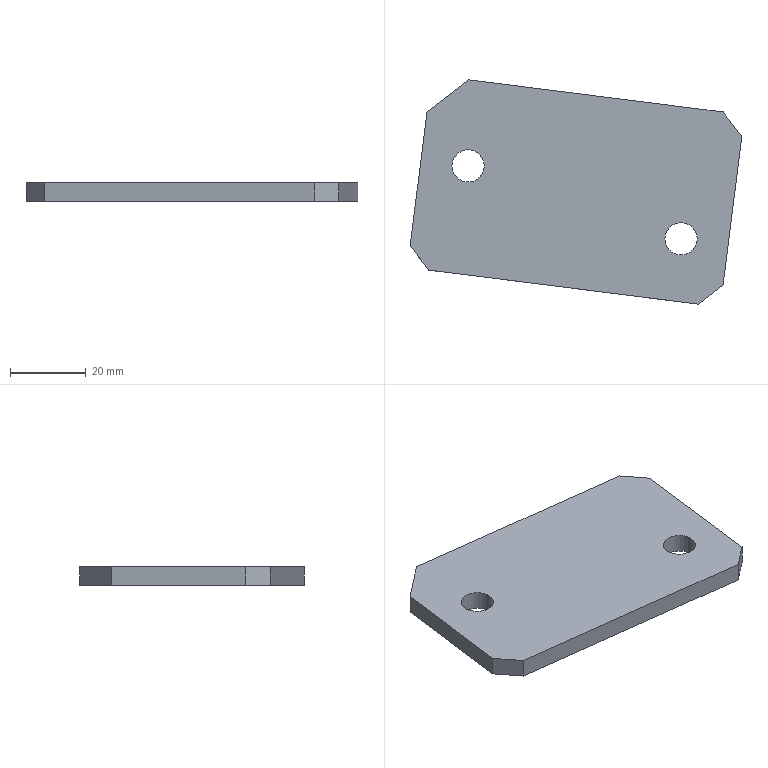Part | STEP file | gslz 2016.10.28-13_id1706_x_t | 1 solid | 12 faces | box 87.307 x 59.069 x 5 mm | volume 20118 mm3 | plane 10 | cylinder 2 | commonest cylinder face diameters 8.5 x2
STEP:
#1=CARTESIAN_POINT('',(0.,0.,0.));
#2=DIRECTION('',(0.,0.,1.));
#3=DIRECTION('',(1.,0.,0.));
#4=AXIS2_PLACEMENT_3D('',#1,#2,#3);
#5=CARTESIAN_POINT('',(33.844,160.175,-99.));
#6=VERTEX_POINT('',#5);
#7=CARTESIAN_POINT('',(-37.177,169.147,-99.));
#8=VERTEX_POINT('',#7);
#9=CARTESIAN_POINT('',(-1593.802,365.794,-99.));
#10=DIRECTION('',(-0.9921,0.1253,0.));
#11=VECTOR('',#10,1.);
#12=LINE('',#9,#11);
#13=CARTESIAN_POINT('',(-1593.802,365.794,-99.));
#14=DIRECTION('',(0.1253,0.9921,0.));
#15=DIRECTION('',(-0.9921,0.1253,0.));
#16=AXIS2_PLACEMENT_3D('',#13,#14,#15);
#17=PLANE('',#16);
#18=CARTESIAN_POINT('',(0.,0.));
#19=DIRECTION('',(1.,0.));
#20=VECTOR('',#19,1.);
#21=LINE('',#18,#20);
#22=(GEOMETRIC_REPRESENTATION_CONTEXT(2)PARAMETRIC_REPRESENTATION_CONTEXT()REPRESENTATION_CONTEXT('',''));
#23=DEFINITIONAL_REPRESENTATION('',(#21),#22);
#24=PCURVE('',#17,#23);
#25=CARTESIAN_POINT('',(-1586.721,421.848,-99.));
#26=DIRECTION('',(0.,0.,1.));
#27=DIRECTION('',(1.,0.,0.));
#28=AXIS2_PLACEMENT_3D('',#25,#26,#27);
#29=PLANE('',#28);
#30=CARTESIAN_POINT('',(-7.081,-56.054));
#31=DIRECTION('',(-0.9921,0.1253));
#32=VECTOR('',#31,1.);
#33=LINE('',#30,#32);
#34=(GEOMETRIC_REPRESENTATION_CONTEXT(2)PARAMETRIC_REPRESENTATION_CONTEXT()REPRESENTATION_CONTEXT('',''));
#35=DEFINITIONAL_REPRESENTATION('',(#33),#34);
#36=PCURVE('',#29,#35);
#37=SURFACE_CURVE('',#12,(#24,#36),.PCURVE_S1.);
#38=EDGE_CURVE('',#6,#8,#37,.T.);
#39=ORIENTED_EDGE('',*,*,#38,.F.);
#40=CARTESIAN_POINT('',(33.844,160.175,-94.));
#41=VERTEX_POINT('',#40);
#42=CARTESIAN_POINT('',(33.844,160.175,-99.));
#43=DIRECTION('',(0.,0.,1.));
#44=VECTOR('',#43,1.);
#45=LINE('',#42,#44);
#46=CARTESIAN_POINT('',(-1640.583,0.));
#47=DIRECTION('',(0.,1.));
#48=VECTOR('',#47,1.);
#49=LINE('',#46,#48);
#50=(GEOMETRIC_REPRESENTATION_CONTEXT(2)PARAMETRIC_REPRESENTATION_CONTEXT()REPRESENTATION_CONTEXT('',''));
#51=DEFINITIONAL_REPRESENTATION('',(#49),#50);
#52=PCURVE('',#17,#51);
#53=CARTESIAN_POINT('',(33.681,160.048,-99.));
#54=DIRECTION('',(-0.6129,0.7902,0.));
#55=DIRECTION('',(0.,0.,1.));
#56=AXIS2_PLACEMENT_3D('',#53,#54,#55);
#57=PLANE('',#56);
#58=CARTESIAN_POINT('',(0.,0.2071));
#59=DIRECTION('',(1.,0.));
#60=VECTOR('',#59,1.);
#61=LINE('',#58,#60);
#62=(GEOMETRIC_REPRESENTATION_CONTEXT(2)PARAMETRIC_REPRESENTATION_CONTEXT()REPRESENTATION_CONTEXT('',''));
#63=DEFINITIONAL_REPRESENTATION('',(#61),#62);
#64=PCURVE('',#57,#63);
#65=SURFACE_CURVE('',#45,(#52,#64),.PCURVE_S1.);
#66=EDGE_CURVE('',#6,#41,#65,.T.);
#67=ORIENTED_EDGE('',*,*,#66,.T.);
#68=CARTESIAN_POINT('',(-37.177,169.147,-94.));
#69=VERTEX_POINT('',#68);
#70=CARTESIAN_POINT('',(-1593.802,365.794,-94.));
#71=DIRECTION('',(-0.9921,0.1253,0.));
#72=VECTOR('',#71,1.);
#73=LINE('',#70,#72);
#74=CARTESIAN_POINT('',(0.,5.));
#75=DIRECTION('',(1.,0.));
#76=VECTOR('',#75,1.);
#77=LINE('',#74,#76);
#78=(GEOMETRIC_REPRESENTATION_CONTEXT(2)PARAMETRIC_REPRESENTATION_CONTEXT()REPRESENTATION_CONTEXT('',''));
#79=DEFINITIONAL_REPRESENTATION('',(#77),#78);
#80=PCURVE('',#17,#79);
#81=CARTESIAN_POINT('',(-1586.721,421.848,-94.));
#82=DIRECTION('',(0.,0.,1.));
#83=DIRECTION('',(1.,0.,0.));
#84=AXIS2_PLACEMENT_3D('',#81,#82,#83);
#85=PLANE('',#84);
#86=CARTESIAN_POINT('',(-7.081,-56.054));
#87=DIRECTION('',(-0.9921,0.1253));
#88=VECTOR('',#87,1.);
#89=LINE('',#86,#88);
#90=(GEOMETRIC_REPRESENTATION_CONTEXT(2)PARAMETRIC_REPRESENTATION_CONTEXT()REPRESENTATION_CONTEXT('',''));
#91=DEFINITIONAL_REPRESENTATION('',(#89),#90);
#92=PCURVE('',#85,#91);
#93=SURFACE_CURVE('',#73,(#80,#92),.PCURVE_S1.);
#94=EDGE_CURVE('',#41,#69,#93,.T.);
#95=ORIENTED_EDGE('',*,*,#94,.T.);
#96=CARTESIAN_POINT('',(-37.177,169.147,-99.));
#97=DIRECTION('',(0.,0.,-1.));
#98=VECTOR('',#97,1.);
#99=LINE('',#96,#98);
#100=CARTESIAN_POINT('',(-1568.997,0.));
#101=DIRECTION('',(0.,-1.));
#102=VECTOR('',#101,1.);
#103=LINE('',#100,#102);
#104=(GEOMETRIC_REPRESENTATION_CONTEXT(2)PARAMETRIC_REPRESENTATION_CONTEXT()REPRESENTATION_CONTEXT('',''));
#105=DEFINITIONAL_REPRESENTATION('',(#103),#104);
#106=PCURVE('',#17,#105);
#107=CARTESIAN_POINT('',(-42.251,175.688,-99.));
#108=DIRECTION('',(-0.7902,-0.6129,0.));
#109=DIRECTION('',(0.,0.,-1.));
#110=AXIS2_PLACEMENT_3D('',#107,#108,#109);
#111=PLANE('',#110);
#112=CARTESIAN_POINT('',(0.,8.278));
#113=DIRECTION('',(1.,0.));
#114=VECTOR('',#113,1.);
#115=LINE('',#112,#114);
#116=(GEOMETRIC_REPRESENTATION_CONTEXT(2)PARAMETRIC_REPRESENTATION_CONTEXT()REPRESENTATION_CONTEXT('',''));
#117=DEFINITIONAL_REPRESENTATION('',(#115),#116);
#118=PCURVE('',#111,#117);
#119=SURFACE_CURVE('',#99,(#106,#118),.PCURVE_S1.);
#120=EDGE_CURVE('',#69,#8,#119,.T.);
#121=ORIENTED_EDGE('',*,*,#120,.T.);
#122=EDGE_LOOP('',(#39,#67,#95,#121));
#123=FACE_BOUND('',#122,.T.);
#124=ADVANCED_FACE('',(#123),#17,.F.);
#125=CARTESIAN_POINT('',(-37.664,210.829,-94.));
#126=VERTEX_POINT('',#125);
#127=CARTESIAN_POINT('',(-42.124,175.524,-94.));
#128=VERTEX_POINT('',#127);
#129=CARTESIAN_POINT('',(-35.758,225.916,-94.));
#130=DIRECTION('',(-0.1253,-0.9921,0.));
#131=VECTOR('',#130,1.);
#132=LINE('',#129,#131);
#133=CARTESIAN_POINT('',(-35.758,225.916,-99.));
#134=DIRECTION('',(-0.9921,0.1253,0.));
#135=DIRECTION('',(-0.1253,-0.9921,0.));
#136=AXIS2_PLACEMENT_3D('',#133,#134,#135);
#137=PLANE('',#136);
#138=CARTESIAN_POINT('',(0.,5.));
#139=DIRECTION('',(1.,0.));
#140=VECTOR('',#139,1.);
#141=LINE('',#138,#140);
#142=(GEOMETRIC_REPRESENTATION_CONTEXT(2)PARAMETRIC_REPRESENTATION_CONTEXT()REPRESENTATION_CONTEXT('',''));
#143=DEFINITIONAL_REPRESENTATION('',(#141),#142);
#144=PCURVE('',#137,#143);
#145=CARTESIAN_POINT('',(1550.963,-195.932));
#146=DIRECTION('',(-0.1253,-0.9921));
#147=VECTOR('',#146,1.);
#148=LINE('',#145,#147);
#149=(GEOMETRIC_REPRESENTATION_CONTEXT(2)PARAMETRIC_REPRESENTATION_CONTEXT()REPRESENTATION_CONTEXT('',''));
#150=DEFINITIONAL_REPRESENTATION('',(#148),#149);
#151=PCURVE('',#85,#150);
#152=SURFACE_CURVE('',#132,(#144,#151),.PCURVE_S1.);
#153=EDGE_CURVE('',#126,#128,#152,.T.);
#154=ORIENTED_EDGE('',*,*,#153,.F.);
#155=CARTESIAN_POINT('',(-37.664,210.829,-99.));
#156=VERTEX_POINT('',#155);
#157=CARTESIAN_POINT('',(-37.664,210.829,-99.));
#158=DIRECTION('',(0.,0.,-1.));
#159=VECTOR('',#158,1.);
#160=LINE('',#157,#159);
#161=CARTESIAN_POINT('',(15.207,0.));
#162=DIRECTION('',(0.,-1.));
#163=VECTOR('',#162,1.);
#164=LINE('',#161,#163);
#165=(GEOMETRIC_REPRESENTATION_CONTEXT(2)PARAMETRIC_REPRESENTATION_CONTEXT()REPRESENTATION_CONTEXT('',''));
#166=DEFINITIONAL_REPRESENTATION('',(#164),#165);
#167=PCURVE('',#137,#166);
#168=CARTESIAN_POINT('',(-26.653,219.37,-99.));
#169=DIRECTION('',(0.6129,-0.7902,0.));
#170=DIRECTION('',(0.,0.,1.));
#171=AXIS2_PLACEMENT_3D('',#168,#169,#170);
#172=PLANE('',#171);
#173=CARTESIAN_POINT('',(0.,13.935));
#174=DIRECTION('',(-1.,0.));
#175=VECTOR('',#174,1.);
#176=LINE('',#173,#175);
#177=(GEOMETRIC_REPRESENTATION_CONTEXT(2)PARAMETRIC_REPRESENTATION_CONTEXT()REPRESENTATION_CONTEXT('',''));
#178=DEFINITIONAL_REPRESENTATION('',(#176),#177);
#179=PCURVE('',#172,#178);
#180=SURFACE_CURVE('',#160,(#167,#179),.PCURVE_S1.);
#181=EDGE_CURVE('',#126,#156,#180,.T.);
#182=ORIENTED_EDGE('',*,*,#181,.T.);
#183=CARTESIAN_POINT('',(-42.124,175.524,-99.));
#184=VERTEX_POINT('',#183);
#185=CARTESIAN_POINT('',(-35.758,225.916,-99.));
#186=DIRECTION('',(-0.1253,-0.9921,0.));
#187=VECTOR('',#186,1.);
#188=LINE('',#185,#187);
#189=CARTESIAN_POINT('',(0.,0.));
#190=DIRECTION('',(1.,0.));
#191=VECTOR('',#190,1.);
#192=LINE('',#189,#191);
#193=(GEOMETRIC_REPRESENTATION_CONTEXT(2)PARAMETRIC_REPRESENTATION_CONTEXT()REPRESENTATION_CONTEXT('',''));
#194=DEFINITIONAL_REPRESENTATION('',(#192),#193);
#195=PCURVE('',#137,#194);
#196=CARTESIAN_POINT('',(1550.963,-195.932));
#197=DIRECTION('',(-0.1253,-0.9921));
#198=VECTOR('',#197,1.);
#199=LINE('',#196,#198);
#200=(GEOMETRIC_REPRESENTATION_CONTEXT(2)PARAMETRIC_REPRESENTATION_CONTEXT()REPRESENTATION_CONTEXT('',''));
#201=DEFINITIONAL_REPRESENTATION('',(#199),#200);
#202=PCURVE('',#29,#201);
#203=SURFACE_CURVE('',#188,(#195,#202),.PCURVE_S1.);
#204=EDGE_CURVE('',#156,#184,#203,.T.);
#205=ORIENTED_EDGE('',*,*,#204,.T.);
#206=CARTESIAN_POINT('',(-42.124,175.524,-99.));
#207=DIRECTION('',(0.,0.,1.));
#208=VECTOR('',#207,1.);
#209=LINE('',#206,#208);
#210=CARTESIAN_POINT('',(50.793,0.));
#211=DIRECTION('',(0.,1.));
#212=VECTOR('',#211,1.);
#213=LINE('',#210,#212);
#214=(GEOMETRIC_REPRESENTATION_CONTEXT(2)PARAMETRIC_REPRESENTATION_CONTEXT()REPRESENTATION_CONTEXT('',''));
#215=DEFINITIONAL_REPRESENTATION('',(#213),#214);
#216=PCURVE('',#137,#215);
#217=CARTESIAN_POINT('',(0.,0.2071));
#218=DIRECTION('',(-1.,0.));
#219=VECTOR('',#218,1.);
#220=LINE('',#217,#219);
#221=(GEOMETRIC_REPRESENTATION_CONTEXT(2)PARAMETRIC_REPRESENTATION_CONTEXT()REPRESENTATION_CONTEXT('',''));
#222=DEFINITIONAL_REPRESENTATION('',(#220),#221);
#223=PCURVE('',#111,#222);
#224=SURFACE_CURVE('',#209,(#216,#223),.PCURVE_S1.);
#225=EDGE_CURVE('',#184,#128,#224,.T.);
#226=ORIENTED_EDGE('',*,*,#225,.T.);
#227=EDGE_LOOP('',(#154,#182,#205,#226));
#228=FACE_BOUND('',#227,.T.);
#229=ADVANCED_FACE('',(#228),#137,.T.);
#230=CARTESIAN_POINT('',(40.236,210.772,-99.));
#231=VERTEX_POINT('',#230);
#232=CARTESIAN_POINT('',(-26.816,219.243,-99.));
#233=VERTEX_POINT('',#232);
#234=CARTESIAN_POINT('',(-1587.41,416.392,-99.));
#235=DIRECTION('',(-0.9921,0.1253,0.));
#236=VECTOR('',#235,1.);
#237=LINE('',#234,#236);
#238=CARTESIAN_POINT('',(-1587.41,416.392,-99.));
#239=DIRECTION('',(0.1253,0.9921,0.));
#240=DIRECTION('',(-0.9921,0.1253,0.));
#241=AXIS2_PLACEMENT_3D('',#238,#239,#240);
#242=PLANE('',#241);
#243=CARTESIAN_POINT('',(0.,0.));
#244=DIRECTION('',(1.,0.));
#245=VECTOR('',#244,1.);
#246=LINE('',#243,#245);
#247=(GEOMETRIC_REPRESENTATION_CONTEXT(2)PARAMETRIC_REPRESENTATION_CONTEXT()REPRESENTATION_CONTEXT('',''));
#248=DEFINITIONAL_REPRESENTATION('',(#246),#247);
#249=PCURVE('',#242,#248);
#250=CARTESIAN_POINT('',(-0.6893,-5.457));
#251=DIRECTION('',(-0.9921,0.1253));
#252=VECTOR('',#251,1.);
#253=LINE('',#250,#252);
#254=(GEOMETRIC_REPRESENTATION_CONTEXT(2)PARAMETRIC_REPRESENTATION_CONTEXT()REPRESENTATION_CONTEXT('',''));
#255=DEFINITIONAL_REPRESENTATION('',(#253),#254);
#256=PCURVE('',#29,#255);
#257=SURFACE_CURVE('',#237,(#249,#256),.PCURVE_S1.);
#258=EDGE_CURVE('',#231,#233,#257,.T.);
#259=ORIENTED_EDGE('',*,*,#258,.T.);
#260=CARTESIAN_POINT('',(-26.816,219.243,-94.));
#261=VERTEX_POINT('',#260);
#262=CARTESIAN_POINT('',(-26.816,219.243,-99.));
#263=DIRECTION('',(0.,0.,1.));
#264=VECTOR('',#263,1.);
#265=LINE('',#262,#264);
#266=CARTESIAN_POINT('',(-1572.997,0.));
#267=DIRECTION('',(0.,1.));
#268=VECTOR('',#267,1.);
#269=LINE('',#266,#268);
#270=(GEOMETRIC_REPRESENTATION_CONTEXT(2)PARAMETRIC_REPRESENTATION_CONTEXT()REPRESENTATION_CONTEXT('',''));
#271=DEFINITIONAL_REPRESENTATION('',(#269),#270);
#272=PCURVE('',#242,#271);
#273=CARTESIAN_POINT('',(0.,0.2071));
#274=DIRECTION('',(1.,0.));
#275=VECTOR('',#274,1.);
#276=LINE('',#273,#275);
#277=(GEOMETRIC_REPRESENTATION_CONTEXT(2)PARAMETRIC_REPRESENTATION_CONTEXT()REPRESENTATION_CONTEXT('',''));
#278=DEFINITIONAL_REPRESENTATION('',(#276),#277);
#279=PCURVE('',#172,#278);
#280=SURFACE_CURVE('',#265,(#272,#279),.PCURVE_S1.);
#281=EDGE_CURVE('',#233,#261,#280,.T.);
#282=ORIENTED_EDGE('',*,*,#281,.T.);
#283=CARTESIAN_POINT('',(40.236,210.772,-94.));
#284=VERTEX_POINT('',#283);
#285=CARTESIAN_POINT('',(-1587.41,416.392,-94.));
#286=DIRECTION('',(-0.9921,0.1253,0.));
#287=VECTOR('',#286,1.);
#288=LINE('',#285,#287);
#289=CARTESIAN_POINT('',(0.,5.));
#290=DIRECTION('',(1.,0.));
#291=VECTOR('',#290,1.);
#292=LINE('',#289,#291);
#293=(GEOMETRIC_REPRESENTATION_CONTEXT(2)PARAMETRIC_REPRESENTATION_CONTEXT()REPRESENTATION_CONTEXT('',''));
#294=DEFINITIONAL_REPRESENTATION('',(#292),#293);
#295=PCURVE('',#242,#294);
#296=CARTESIAN_POINT('',(-0.6893,-5.457));
#297=DIRECTION('',(-0.9921,0.1253));
#298=VECTOR('',#297,1.);
#299=LINE('',#296,#298);
#300=(GEOMETRIC_REPRESENTATION_CONTEXT(2)PARAMETRIC_REPRESENTATION_CONTEXT()REPRESENTATION_CONTEXT('',''));
#301=DEFINITIONAL_REPRESENTATION('',(#299),#300);
#302=PCURVE('',#85,#301);
#303=SURFACE_CURVE('',#288,(#295,#302),.PCURVE_S1.);
#304=EDGE_CURVE('',#284,#261,#303,.T.);
#305=ORIENTED_EDGE('',*,*,#304,.F.);
#306=CARTESIAN_POINT('',(40.236,210.772,-99.));
#307=DIRECTION('',(0.,0.,-1.));
#308=VECTOR('',#307,1.);
#309=LINE('',#306,#308);
#310=CARTESIAN_POINT('',(-1640.583,0.));
#311=DIRECTION('',(0.,-1.));
#312=VECTOR('',#311,1.);
#313=LINE('',#310,#312);
#314=(GEOMETRIC_REPRESENTATION_CONTEXT(2)PARAMETRIC_REPRESENTATION_CONTEXT()REPRESENTATION_CONTEXT('',''));
#315=DEFINITIONAL_REPRESENTATION('',(#313),#314);
#316=PCURVE('',#242,#315);
#317=CARTESIAN_POINT('',(45.31,204.231,-99.));
#318=DIRECTION('',(0.7902,0.6129,0.));
#319=DIRECTION('',(0.,0.,-1.));
#320=AXIS2_PLACEMENT_3D('',#317,#318,#319);
#321=PLANE('',#320);
#322=CARTESIAN_POINT('',(0.,8.278));
#323=DIRECTION('',(1.,0.));
#324=VECTOR('',#323,1.);
#325=LINE('',#322,#324);
#326=(GEOMETRIC_REPRESENTATION_CONTEXT(2)PARAMETRIC_REPRESENTATION_CONTEXT()REPRESENTATION_CONTEXT('',''));
#327=DEFINITIONAL_REPRESENTATION('',(#325),#326);
#328=PCURVE('',#321,#327);
#329=SURFACE_CURVE('',#309,(#316,#328),.PCURVE_S1.);
#330=EDGE_CURVE('',#284,#231,#329,.T.);
#331=ORIENTED_EDGE('',*,*,#330,.T.);
#332=EDGE_LOOP('',(#259,#282,#305,#331));
#333=FACE_BOUND('',#332,.T.);
#334=ADVANCED_FACE('',(#333),#242,.T.);
#335=CARTESIAN_POINT('',(45.183,204.395,-99.));
#336=VERTEX_POINT('',#335);
#337=CARTESIAN_POINT('',(40.222,165.121,-99.));
#338=VERTEX_POINT('',#337);
#339=CARTESIAN_POINT('',(46.588,215.514,-99.));
#340=DIRECTION('',(-0.1253,-0.9921,0.));
#341=VECTOR('',#340,1.);
#342=LINE('',#339,#341);
#343=CARTESIAN_POINT('',(46.588,215.514,-99.));
#344=DIRECTION('',(-0.9921,0.1253,0.));
#345=DIRECTION('',(-0.1253,-0.9921,0.));
#346=AXIS2_PLACEMENT_3D('',#343,#344,#345);
#347=PLANE('',#346);
#348=CARTESIAN_POINT('',(0.,0.));
#349=DIRECTION('',(1.,0.));
#350=VECTOR('',#349,1.);
#351=LINE('',#348,#350);
#352=(GEOMETRIC_REPRESENTATION_CONTEXT(2)PARAMETRIC_REPRESENTATION_CONTEXT()REPRESENTATION_CONTEXT('',''));
#353=DEFINITIONAL_REPRESENTATION('',(#351),#352);
#354=PCURVE('',#347,#353);
#355=CARTESIAN_POINT('',(1633.309,-206.334));
#356=DIRECTION('',(-0.1253,-0.9921));
#357=VECTOR('',#356,1.);
#358=LINE('',#355,#357);
#359=(GEOMETRIC_REPRESENTATION_CONTEXT(2)PARAMETRIC_REPRESENTATION_CONTEXT()REPRESENTATION_CONTEXT('',''));
#360=DEFINITIONAL_REPRESENTATION('',(#358),#359);
#361=PCURVE('',#29,#360);
#362=SURFACE_CURVE('',#342,(#354,#361),.PCURVE_S1.);
#363=EDGE_CURVE('',#336,#338,#362,.T.);
#364=ORIENTED_EDGE('',*,*,#363,.F.);
#365=CARTESIAN_POINT('',(45.183,204.395,-94.));
#366=VERTEX_POINT('',#365);
#367=CARTESIAN_POINT('',(45.183,204.395,-99.));
#368=DIRECTION('',(0.,0.,1.));
#369=VECTOR('',#368,1.);
#370=LINE('',#367,#369);
#371=CARTESIAN_POINT('',(11.207,0.));
#372=DIRECTION('',(0.,1.));
#373=VECTOR('',#372,1.);
#374=LINE('',#371,#373);
#375=(GEOMETRIC_REPRESENTATION_CONTEXT(2)PARAMETRIC_REPRESENTATION_CONTEXT()REPRESENTATION_CONTEXT('',''));
#376=DEFINITIONAL_REPRESENTATION('',(#374),#375);
#377=PCURVE('',#347,#376);
#378=CARTESIAN_POINT('',(0.,0.2071));
#379=DIRECTION('',(-1.,0.));
#380=VECTOR('',#379,1.);
#381=LINE('',#378,#380);
#382=(GEOMETRIC_REPRESENTATION_CONTEXT(2)PARAMETRIC_REPRESENTATION_CONTEXT()REPRESENTATION_CONTEXT('',''));
#383=DEFINITIONAL_REPRESENTATION('',(#381),#382);
#384=PCURVE('',#321,#383);
#385=SURFACE_CURVE('',#370,(#377,#384),.PCURVE_S1.);
#386=EDGE_CURVE('',#336,#366,#385,.T.);
#387=ORIENTED_EDGE('',*,*,#386,.T.);
#388=CARTESIAN_POINT('',(40.222,165.121,-94.));
#389=VERTEX_POINT('',#388);
#390=CARTESIAN_POINT('',(46.588,215.514,-94.));
#391=DIRECTION('',(-0.1253,-0.9921,0.));
#392=VECTOR('',#391,1.);
#393=LINE('',#390,#392);
#394=CARTESIAN_POINT('',(0.,5.));
#395=DIRECTION('',(1.,0.));
#396=VECTOR('',#395,1.);
#397=LINE('',#394,#396);
#398=(GEOMETRIC_REPRESENTATION_CONTEXT(2)PARAMETRIC_REPRESENTATION_CONTEXT()REPRESENTATION_CONTEXT('',''));
#399=DEFINITIONAL_REPRESENTATION('',(#397),#398);
#400=PCURVE('',#347,#399);
#401=CARTESIAN_POINT('',(1633.309,-206.334));
#402=DIRECTION('',(-0.1253,-0.9921));
#403=VECTOR('',#402,1.);
#404=LINE('',#401,#403);
#405=(GEOMETRIC_REPRESENTATION_CONTEXT(2)PARAMETRIC_REPRESENTATION_CONTEXT()REPRESENTATION_CONTEXT('',''));
#406=DEFINITIONAL_REPRESENTATION('',(#404),#405);
#407=PCURVE('',#85,#406);
#408=SURFACE_CURVE('',#393,(#400,#407),.PCURVE_S1.);
#409=EDGE_CURVE('',#366,#389,#408,.T.);
#410=ORIENTED_EDGE('',*,*,#409,.T.);
#411=CARTESIAN_POINT('',(40.222,165.121,-99.));
#412=DIRECTION('',(0.,0.,-1.));
#413=VECTOR('',#412,1.);
#414=LINE('',#411,#413);
#415=CARTESIAN_POINT('',(50.793,0.));
#416=DIRECTION('',(0.,-1.));
#417=VECTOR('',#416,1.);
#418=LINE('',#415,#417);
#419=(GEOMETRIC_REPRESENTATION_CONTEXT(2)PARAMETRIC_REPRESENTATION_CONTEXT()REPRESENTATION_CONTEXT('',''));
#420=DEFINITIONAL_REPRESENTATION('',(#418),#419);
#421=PCURVE('',#347,#420);
#422=CARTESIAN_POINT('',(0.,8.278));
#423=DIRECTION('',(-1.,0.));
#424=VECTOR('',#423,1.);
#425=LINE('',#422,#424);
#426=(GEOMETRIC_REPRESENTATION_CONTEXT(2)PARAMETRIC_REPRESENTATION_CONTEXT()REPRESENTATION_CONTEXT('',''));
#427=DEFINITIONAL_REPRESENTATION('',(#425),#426);
#428=PCURVE('',#57,#427);
#429=SURFACE_CURVE('',#414,(#421,#428),.PCURVE_S1.);
#430=EDGE_CURVE('',#389,#338,#429,.T.);
#431=ORIENTED_EDGE('',*,*,#430,.T.);
#432=EDGE_LOOP('',(#364,#387,#410,#431));
#433=FACE_BOUND('',#432,.T.);
#434=ADVANCED_FACE('',(#433),#347,.F.);
#435=CARTESIAN_POINT('',(-31.116,196.571,-99.));
#436=VERTEX_POINT('',#435);
#437=CARTESIAN_POINT('',(-26.866,196.571,-99.));
#438=DIRECTION('',(0.,0.,-1.));
#439=DIRECTION('',(-1.,0.,0.));
#440=AXIS2_PLACEMENT_3D('',#437,#438,#439);
#441=CIRCLE('',#440,4.25);
#442=CARTESIAN_POINT('',(-26.866,196.571,-99.));
#443=DIRECTION('',(0.,0.,1.));
#444=DIRECTION('',(1.,0.,0.));
#445=AXIS2_PLACEMENT_3D('',#442,#443,#444);
#446=CYLINDRICAL_SURFACE('',#445,4.25);
#447=CARTESIAN_POINT('',(9.425,0.));
#448=DIRECTION('',(-1.,0.));
#449=VECTOR('',#448,1.);
#450=LINE('',#447,#449);
#451=(GEOMETRIC_REPRESENTATION_CONTEXT(2)PARAMETRIC_REPRESENTATION_CONTEXT()REPRESENTATION_CONTEXT('',''));
#452=DEFINITIONAL_REPRESENTATION('',(#450),#451);
#453=PCURVE('',#446,#452);
#454=CARTESIAN_POINT('',(1555.605,-225.278));
#455=CARTESIAN_POINT('',(1555.605,-217.916));
#456=CARTESIAN_POINT('',(1561.98,-221.597));
#457=CARTESIAN_POINT('',(1568.355,-225.278));
#458=CARTESIAN_POINT('',(1561.98,-228.958));
#459=CARTESIAN_POINT('',(1555.605,-232.639));
#460=CARTESIAN_POINT('',(1555.605,-225.278));
#461=(BOUNDED_CURVE()B_SPLINE_CURVE(2,(#454,#455,#456,#457,#458,#459,#460),.UNSPECIFIED.,.T.,.F.)B_SPLINE_CURVE_WITH_KNOTS((1,2,2,2,2,1),(-2.094,0.,2.094,4.189,6.283,8.378),.UNSPECIFIED.)CURVE()GEOMETRIC_REPRESENTATION_ITEM()RATIONAL_B_SPLINE_CURVE((1.,0.5,1.,0.5,1.,0.5,1.))REPRESENTATION_ITEM(''));
#462=(GEOMETRIC_REPRESENTATION_CONTEXT(2)PARAMETRIC_REPRESENTATION_CONTEXT()REPRESENTATION_CONTEXT('',''));
#463=DEFINITIONAL_REPRESENTATION('',(#461),#462);
#464=PCURVE('',#29,#463);
#465=SURFACE_CURVE('',#441,(#453,#464),.PCURVE_S1.);
#466=EDGE_CURVE('',#436,#436,#465,.T.);
#467=ORIENTED_EDGE('',*,*,#466,.F.);
#468=CARTESIAN_POINT('',(-31.116,196.571,-94.));
#469=VERTEX_POINT('',#468);
#470=CARTESIAN_POINT('',(-31.116,196.571,-99.));
#471=CARTESIAN_POINT('',(-31.116,196.571,-94.));
#472=B_SPLINE_CURVE_WITH_KNOTS('',1,(#470,#471),.UNSPECIFIED.,.F.,.F.,(2,2),(0.,5.),.PIECEWISE_BEZIER_KNOTS.);
#473=CARTESIAN_POINT('',(9.425,0.));
#474=DIRECTION('',(0.,1.));
#475=VECTOR('',#474,1.);
#476=LINE('',#473,#475);
#477=(GEOMETRIC_REPRESENTATION_CONTEXT(2)PARAMETRIC_REPRESENTATION_CONTEXT()REPRESENTATION_CONTEXT('',''));
#478=DEFINITIONAL_REPRESENTATION('',(#476),#477);
#479=PCURVE('',#446,#478);
#480=CARTESIAN_POINT('',(3.142,0.));
#481=DIRECTION('',(0.,1.));
#482=VECTOR('',#481,1.);
#483=LINE('',#480,#482);
#484=(GEOMETRIC_REPRESENTATION_CONTEXT(2)PARAMETRIC_REPRESENTATION_CONTEXT()REPRESENTATION_CONTEXT('',''));
#485=DEFINITIONAL_REPRESENTATION('',(#483),#484);
#486=PCURVE('',#446,#485);
#487=SEAM_CURVE('',#472,(#479,#486),.PCURVE_S1.);
#488=EDGE_CURVE('',#436,#469,#487,.T.);
#489=ORIENTED_EDGE('',*,*,#488,.T.);
#490=CARTESIAN_POINT('',(-26.866,196.571,-94.));
#491=DIRECTION('',(0.,0.,-1.));
#492=DIRECTION('',(-1.,0.,0.));
#493=AXIS2_PLACEMENT_3D('',#490,#491,#492);
#494=CIRCLE('',#493,4.25);
#495=CARTESIAN_POINT('',(9.425,5.));
#496=DIRECTION('',(-1.,0.));
#497=VECTOR('',#496,1.);
#498=LINE('',#495,#497);
#499=(GEOMETRIC_REPRESENTATION_CONTEXT(2)PARAMETRIC_REPRESENTATION_CONTEXT()REPRESENTATION_CONTEXT('',''));
#500=DEFINITIONAL_REPRESENTATION('',(#498),#499);
#501=PCURVE('',#446,#500);
#502=CARTESIAN_POINT('',(1555.605,-225.278));
#503=CARTESIAN_POINT('',(1555.605,-217.916));
#504=CARTESIAN_POINT('',(1561.98,-221.597));
#505=CARTESIAN_POINT('',(1568.355,-225.278));
#506=CARTESIAN_POINT('',(1561.98,-228.958));
#507=CARTESIAN_POINT('',(1555.605,-232.639));
#508=CARTESIAN_POINT('',(1555.605,-225.278));
#509=(BOUNDED_CURVE()B_SPLINE_CURVE(2,(#502,#503,#504,#505,#506,#507,#508),.UNSPECIFIED.,.T.,.F.)B_SPLINE_CURVE_WITH_KNOTS((1,2,2,2,2,1),(-2.094,0.,2.094,4.189,6.283,8.378),.UNSPECIFIED.)CURVE()GEOMETRIC_REPRESENTATION_ITEM()RATIONAL_B_SPLINE_CURVE((1.,0.5,1.,0.5,1.,0.5,1.))REPRESENTATION_ITEM(''));
#510=(GEOMETRIC_REPRESENTATION_CONTEXT(2)PARAMETRIC_REPRESENTATION_CONTEXT()REPRESENTATION_CONTEXT('',''));
#511=DEFINITIONAL_REPRESENTATION('',(#509),#510);
#512=PCURVE('',#85,#511);
#513=SURFACE_CURVE('',#494,(#501,#512),.PCURVE_S1.);
#514=EDGE_CURVE('',#469,#469,#513,.T.);
#515=ORIENTED_EDGE('',*,*,#514,.T.);
#516=ORIENTED_EDGE('',*,*,#488,.F.);
#517=EDGE_LOOP('',(#467,#489,#515,#516));
#518=FACE_BOUND('',#517,.F.);
#519=ADVANCED_FACE('',(#518),#446,.F.);
#520=CARTESIAN_POINT('',(24.923,177.396,-99.));
#521=VERTEX_POINT('',#520);
#522=CARTESIAN_POINT('',(29.173,177.396,-99.));
#523=DIRECTION('',(0.,0.,-1.));
#524=DIRECTION('',(-1.,0.,0.));
#525=AXIS2_PLACEMENT_3D('',#522,#523,#524);
#526=CIRCLE('',#525,4.25);
#527=CARTESIAN_POINT('',(29.173,177.396,-99.));
#528=DIRECTION('',(0.,0.,1.));
#529=DIRECTION('',(1.,0.,0.));
#530=AXIS2_PLACEMENT_3D('',#527,#528,#529);
#531=CYLINDRICAL_SURFACE('',#530,4.25);
#532=CARTESIAN_POINT('',(9.425,0.));
#533=DIRECTION('',(-1.,0.));
#534=VECTOR('',#533,1.);
#535=LINE('',#532,#534);
#536=(GEOMETRIC_REPRESENTATION_CONTEXT(2)PARAMETRIC_REPRESENTATION_CONTEXT()REPRESENTATION_CONTEXT('',''));
#537=DEFINITIONAL_REPRESENTATION('',(#535),#536);
#538=PCURVE('',#531,#537);
#539=CARTESIAN_POINT('',(1611.644,-244.452));
#540=CARTESIAN_POINT('',(1611.644,-237.091));
#541=CARTESIAN_POINT('',(1618.019,-240.772));
#542=CARTESIAN_POINT('',(1624.394,-244.452));
#543=CARTESIAN_POINT('',(1618.019,-248.133));
#544=CARTESIAN_POINT('',(1611.644,-251.814));
#545=CARTESIAN_POINT('',(1611.644,-244.452));
#546=(BOUNDED_CURVE()B_SPLINE_CURVE(2,(#539,#540,#541,#542,#543,#544,#545),.UNSPECIFIED.,.T.,.F.)B_SPLINE_CURVE_WITH_KNOTS((1,2,2,2,2,1),(-2.094,0.,2.094,4.189,6.283,8.378),.UNSPECIFIED.)CURVE()GEOMETRIC_REPRESENTATION_ITEM()RATIONAL_B_SPLINE_CURVE((1.,0.5,1.,0.5,1.,0.5,1.))REPRESENTATION_ITEM(''));
#547=(GEOMETRIC_REPRESENTATION_CONTEXT(2)PARAMETRIC_REPRESENTATION_CONTEXT()REPRESENTATION_CONTEXT('',''));
#548=DEFINITIONAL_REPRESENTATION('',(#546),#547);
#549=PCURVE('',#29,#548);
#550=SURFACE_CURVE('',#526,(#538,#549),.PCURVE_S1.);
#551=EDGE_CURVE('',#521,#521,#550,.T.);
#552=ORIENTED_EDGE('',*,*,#551,.F.);
#553=CARTESIAN_POINT('',(24.923,177.396,-94.));
#554=VERTEX_POINT('',#553);
#555=CARTESIAN_POINT('',(24.923,177.396,-99.));
#556=CARTESIAN_POINT('',(24.923,177.396,-94.));
#557=B_SPLINE_CURVE_WITH_KNOTS('',1,(#555,#556),.UNSPECIFIED.,.F.,.F.,(2,2),(0.,5.),.PIECEWISE_BEZIER_KNOTS.);
#558=CARTESIAN_POINT('',(9.425,0.));
#559=DIRECTION('',(0.,1.));
#560=VECTOR('',#559,1.);
#561=LINE('',#558,#560);
#562=(GEOMETRIC_REPRESENTATION_CONTEXT(2)PARAMETRIC_REPRESENTATION_CONTEXT()REPRESENTATION_CONTEXT('',''));
#563=DEFINITIONAL_REPRESENTATION('',(#561),#562);
#564=PCURVE('',#531,#563);
#565=CARTESIAN_POINT('',(3.142,0.));
#566=DIRECTION('',(0.,1.));
#567=VECTOR('',#566,1.);
#568=LINE('',#565,#567);
#569=(GEOMETRIC_REPRESENTATION_CONTEXT(2)PARAMETRIC_REPRESENTATION_CONTEXT()REPRESENTATION_CONTEXT('',''));
#570=DEFINITIONAL_REPRESENTATION('',(#568),#569);
#571=PCURVE('',#531,#570);
#572=SEAM_CURVE('',#557,(#564,#571),.PCURVE_S1.);
#573=EDGE_CURVE('',#521,#554,#572,.T.);
#574=ORIENTED_EDGE('',*,*,#573,.T.);
#575=CARTESIAN_POINT('',(29.173,177.396,-94.));
#576=DIRECTION('',(0.,0.,-1.));
#577=DIRECTION('',(-1.,0.,0.));
#578=AXIS2_PLACEMENT_3D('',#575,#576,#577);
#579=CIRCLE('',#578,4.25);
#580=CARTESIAN_POINT('',(9.425,5.));
#581=DIRECTION('',(-1.,0.));
#582=VECTOR('',#581,1.);
#583=LINE('',#580,#582);
#584=(GEOMETRIC_REPRESENTATION_CONTEXT(2)PARAMETRIC_REPRESENTATION_CONTEXT()REPRESENTATION_CONTEXT('',''));
#585=DEFINITIONAL_REPRESENTATION('',(#583),#584);
#586=PCURVE('',#531,#585);
#587=CARTESIAN_POINT('',(1611.644,-244.452));
#588=CARTESIAN_POINT('',(1611.644,-237.091));
#589=CARTESIAN_POINT('',(1618.019,-240.772));
#590=CARTESIAN_POINT('',(1624.394,-244.452));
#591=CARTESIAN_POINT('',(1618.019,-248.133));
#592=CARTESIAN_POINT('',(1611.644,-251.814));
#593=CARTESIAN_POINT('',(1611.644,-244.452));
#594=(BOUNDED_CURVE()B_SPLINE_CURVE(2,(#587,#588,#589,#590,#591,#592,#593),.UNSPECIFIED.,.T.,.F.)B_SPLINE_CURVE_WITH_KNOTS((1,2,2,2,2,1),(-2.094,0.,2.094,4.189,6.283,8.378),.UNSPECIFIED.)CURVE()GEOMETRIC_REPRESENTATION_ITEM()RATIONAL_B_SPLINE_CURVE((1.,0.5,1.,0.5,1.,0.5,1.))REPRESENTATION_ITEM(''));
#595=(GEOMETRIC_REPRESENTATION_CONTEXT(2)PARAMETRIC_REPRESENTATION_CONTEXT()REPRESENTATION_CONTEXT('',''));
#596=DEFINITIONAL_REPRESENTATION('',(#594),#595);
#597=PCURVE('',#85,#596);
#598=SURFACE_CURVE('',#579,(#586,#597),.PCURVE_S1.);
#599=EDGE_CURVE('',#554,#554,#598,.T.);
#600=ORIENTED_EDGE('',*,*,#599,.T.);
#601=ORIENTED_EDGE('',*,*,#573,.F.);
#602=EDGE_LOOP('',(#552,#574,#600,#601));
#603=FACE_BOUND('',#602,.F.);
#604=ADVANCED_FACE('',(#603),#531,.F.);
#605=ORIENTED_EDGE('',*,*,#204,.F.);
#606=CARTESIAN_POINT('',(-26.653,219.37,-99.));
#607=DIRECTION('',(0.7902,0.6129,0.));
#608=VECTOR('',#607,1.);
#609=LINE('',#606,#608);
#610=CARTESIAN_POINT('',(1560.068,-202.478));
#611=DIRECTION('',(0.7902,0.6129));
#612=VECTOR('',#611,1.);
#613=LINE('',#610,#612);
#614=(GEOMETRIC_REPRESENTATION_CONTEXT(2)PARAMETRIC_REPRESENTATION_CONTEXT()REPRESENTATION_CONTEXT('',''));
#615=DEFINITIONAL_REPRESENTATION('',(#613),#614);
#616=PCURVE('',#29,#615);
#617=CARTESIAN_POINT('',(0.,0.));
#618=DIRECTION('',(0.,-1.));
#619=VECTOR('',#618,1.);
#620=LINE('',#617,#619);
#621=(GEOMETRIC_REPRESENTATION_CONTEXT(2)PARAMETRIC_REPRESENTATION_CONTEXT()REPRESENTATION_CONTEXT('',''));
#622=DEFINITIONAL_REPRESENTATION('',(#620),#621);
#623=PCURVE('',#172,#622);
#624=SURFACE_CURVE('',#609,(#616,#623),.PCURVE_S1.);
#625=EDGE_CURVE('',#156,#233,#624,.T.);
#626=ORIENTED_EDGE('',*,*,#625,.T.);
#627=ORIENTED_EDGE('',*,*,#258,.F.);
#628=CARTESIAN_POINT('',(45.31,204.231,-99.));
#629=DIRECTION('',(0.6129,-0.7902,0.));
#630=VECTOR('',#629,1.);
#631=LINE('',#628,#630);
#632=CARTESIAN_POINT('',(1632.031,-217.617));
#633=DIRECTION('',(0.6129,-0.7902));
#634=VECTOR('',#633,1.);
#635=LINE('',#632,#634);
#636=(GEOMETRIC_REPRESENTATION_CONTEXT(2)PARAMETRIC_REPRESENTATION_CONTEXT()REPRESENTATION_CONTEXT('',''));
#637=DEFINITIONAL_REPRESENTATION('',(#635),#636);
#638=PCURVE('',#29,#637);
#639=CARTESIAN_POINT('',(0.,0.));
#640=DIRECTION('',(0.,-1.));
#641=VECTOR('',#640,1.);
#642=LINE('',#639,#641);
#643=(GEOMETRIC_REPRESENTATION_CONTEXT(2)PARAMETRIC_REPRESENTATION_CONTEXT()REPRESENTATION_CONTEXT('',''));
#644=DEFINITIONAL_REPRESENTATION('',(#642),#643);
#645=PCURVE('',#321,#644);
#646=SURFACE_CURVE('',#631,(#638,#645),.PCURVE_S1.);
#647=EDGE_CURVE('',#231,#336,#646,.T.);
#648=ORIENTED_EDGE('',*,*,#647,.T.);
#649=ORIENTED_EDGE('',*,*,#363,.T.);
#650=CARTESIAN_POINT('',(33.681,160.048,-99.));
#651=DIRECTION('',(-0.7902,-0.6129,0.));
#652=VECTOR('',#651,1.);
#653=LINE('',#650,#652);
#654=CARTESIAN_POINT('',(1620.402,-261.801));
#655=DIRECTION('',(-0.7902,-0.6129));
#656=VECTOR('',#655,1.);
#657=LINE('',#654,#656);
#658=(GEOMETRIC_REPRESENTATION_CONTEXT(2)PARAMETRIC_REPRESENTATION_CONTEXT()REPRESENTATION_CONTEXT('',''));
#659=DEFINITIONAL_REPRESENTATION('',(#657),#658);
#660=PCURVE('',#29,#659);
#661=CARTESIAN_POINT('',(0.,0.));
#662=DIRECTION('',(0.,-1.));
#663=VECTOR('',#662,1.);
#664=LINE('',#661,#663);
#665=(GEOMETRIC_REPRESENTATION_CONTEXT(2)PARAMETRIC_REPRESENTATION_CONTEXT()REPRESENTATION_CONTEXT('',''));
#666=DEFINITIONAL_REPRESENTATION('',(#664),#665);
#667=PCURVE('',#57,#666);
#668=SURFACE_CURVE('',#653,(#660,#667),.PCURVE_S1.);
#669=EDGE_CURVE('',#338,#6,#668,.T.);
#670=ORIENTED_EDGE('',*,*,#669,.T.);
#671=ORIENTED_EDGE('',*,*,#38,.T.);
#672=CARTESIAN_POINT('',(-42.251,175.688,-99.));
#673=DIRECTION('',(-0.6129,0.7902,0.));
#674=VECTOR('',#673,1.);
#675=LINE('',#672,#674);
#676=CARTESIAN_POINT('',(1544.47,-246.161));
#677=DIRECTION('',(-0.6129,0.7902));
#678=VECTOR('',#677,1.);
#679=LINE('',#676,#678);
#680=(GEOMETRIC_REPRESENTATION_CONTEXT(2)PARAMETRIC_REPRESENTATION_CONTEXT()REPRESENTATION_CONTEXT('',''));
#681=DEFINITIONAL_REPRESENTATION('',(#679),#680);
#682=PCURVE('',#29,#681);
#683=CARTESIAN_POINT('',(0.,0.));
#684=DIRECTION('',(0.,-1.));
#685=VECTOR('',#684,1.);
#686=LINE('',#683,#685);
#687=(GEOMETRIC_REPRESENTATION_CONTEXT(2)PARAMETRIC_REPRESENTATION_CONTEXT()REPRESENTATION_CONTEXT('',''));
#688=DEFINITIONAL_REPRESENTATION('',(#686),#687);
#689=PCURVE('',#111,#688);
#690=SURFACE_CURVE('',#675,(#682,#689),.PCURVE_S1.);
#691=EDGE_CURVE('',#8,#184,#690,.T.);
#692=ORIENTED_EDGE('',*,*,#691,.T.);
#693=EDGE_LOOP('',(#605,#626,#627,#648,#649,#670,#671,#692));
#694=FACE_BOUND('',#693,.T.);
#695=ORIENTED_EDGE('',*,*,#466,.F.);
#696=EDGE_LOOP('',(#695));
#697=FACE_BOUND('',#696,.T.);
#698=ORIENTED_EDGE('',*,*,#551,.F.);
#699=EDGE_LOOP('',(#698));
#700=FACE_BOUND('',#699,.T.);
#701=ADVANCED_FACE('',(#694,#697,#700),#29,.F.);
#702=ORIENTED_EDGE('',*,*,#304,.T.);
#703=CARTESIAN_POINT('',(-902.615,-460.096,-94.));
#704=DIRECTION('',(-0.7902,-0.6129,0.));
#705=VECTOR('',#704,1.);
#706=LINE('',#703,#705);
#707=CARTESIAN_POINT('',(684.106,-881.944));
#708=DIRECTION('',(-0.7902,-0.6129));
#709=VECTOR('',#708,1.);
#710=LINE('',#707,#709);
#711=(GEOMETRIC_REPRESENTATION_CONTEXT(2)PARAMETRIC_REPRESENTATION_CONTEXT()REPRESENTATION_CONTEXT('',''));
#712=DEFINITIONAL_REPRESENTATION('',(#710),#711);
#713=PCURVE('',#85,#712);
#714=CARTESIAN_POINT('',(5.,1108.595));
#715=DIRECTION('',(0.,1.));
#716=VECTOR('',#715,1.);
#717=LINE('',#714,#716);
#718=(GEOMETRIC_REPRESENTATION_CONTEXT(2)PARAMETRIC_REPRESENTATION_CONTEXT()REPRESENTATION_CONTEXT('',''));
#719=DEFINITIONAL_REPRESENTATION('',(#717),#718);
#720=PCURVE('',#172,#719);
#721=SURFACE_CURVE('',#706,(#713,#720),.PCURVE_S1.);
#722=EDGE_CURVE('',#261,#126,#721,.T.);
#723=ORIENTED_EDGE('',*,*,#722,.T.);
#724=ORIENTED_EDGE('',*,*,#153,.T.);
#725=CARTESIAN_POINT('',(-737.752,1072.322,-94.));
#726=DIRECTION('',(0.6129,-0.7902,0.));
#727=VECTOR('',#726,1.);
#728=LINE('',#725,#727);
#729=CARTESIAN_POINT('',(848.969,650.474));
#730=DIRECTION('',(0.6129,-0.7902));
#731=VECTOR('',#730,1.);
#732=LINE('',#729,#731);
#733=(GEOMETRIC_REPRESENTATION_CONTEXT(2)PARAMETRIC_REPRESENTATION_CONTEXT()REPRESENTATION_CONTEXT('',''));
#734=DEFINITIONAL_REPRESENTATION('',(#732),#733);
#735=PCURVE('',#85,#734);
#736=CARTESIAN_POINT('',(-5.,-1134.758));
#737=DIRECTION('',(0.,1.));
#738=VECTOR('',#737,1.);
#739=LINE('',#736,#738);
#740=(GEOMETRIC_REPRESENTATION_CONTEXT(2)PARAMETRIC_REPRESENTATION_CONTEXT()REPRESENTATION_CONTEXT('',''));
#741=DEFINITIONAL_REPRESENTATION('',(#739),#740);
#742=PCURVE('',#111,#741);
#743=SURFACE_CURVE('',#728,(#735,#742),.PCURVE_S1.);
#744=EDGE_CURVE('',#128,#69,#743,.T.);
#745=ORIENTED_EDGE('',*,*,#744,.T.);
#746=ORIENTED_EDGE('',*,*,#94,.F.);
#747=CARTESIAN_POINT('',(-856.249,-530.253,-94.));
#748=DIRECTION('',(0.7902,0.6129,0.));
#749=VECTOR('',#748,1.);
#750=LINE('',#747,#749);
#751=CARTESIAN_POINT('',(730.472,-952.101));
#752=DIRECTION('',(0.7902,0.6129));
#753=VECTOR('',#752,1.);
#754=LINE('',#751,#753);
#755=(GEOMETRIC_REPRESENTATION_CONTEXT(2)PARAMETRIC_REPRESENTATION_CONTEXT()REPRESENTATION_CONTEXT('',''));
#756=DEFINITIONAL_REPRESENTATION('',(#754),#755);
#757=PCURVE('',#85,#756);
#758=CARTESIAN_POINT('',(5.,-1126.273));
#759=DIRECTION('',(0.,1.));
#760=VECTOR('',#759,1.);
#761=LINE('',#758,#760);
#762=(GEOMETRIC_REPRESENTATION_CONTEXT(2)PARAMETRIC_REPRESENTATION_CONTEXT()REPRESENTATION_CONTEXT('',''));
#763=DEFINITIONAL_REPRESENTATION('',(#761),#762);
#764=PCURVE('',#57,#763);
#765=SURFACE_CURVE('',#750,(#757,#764),.PCURVE_S1.);
#766=EDGE_CURVE('',#41,#389,#765,.T.);
#767=ORIENTED_EDGE('',*,*,#766,.T.);
#768=ORIENTED_EDGE('',*,*,#409,.F.);
#769=CARTESIAN_POINT('',(-673.161,1130.478,-94.));
#770=DIRECTION('',(-0.6129,0.7902,0.));
#771=VECTOR('',#770,1.);
#772=LINE('',#769,#771);
#773=CARTESIAN_POINT('',(913.56,708.63));
#774=DIRECTION('',(-0.6129,0.7902));
#775=VECTOR('',#774,1.);
#776=LINE('',#773,#775);
#777=(GEOMETRIC_REPRESENTATION_CONTEXT(2)PARAMETRIC_REPRESENTATION_CONTEXT()REPRESENTATION_CONTEXT('',''));
#778=DEFINITIONAL_REPRESENTATION('',(#776),#777);
#779=PCURVE('',#85,#778);
#780=CARTESIAN_POINT('',(-5.,1172.235));
#781=DIRECTION('',(0.,1.));
#782=VECTOR('',#781,1.);
#783=LINE('',#780,#782);
#784=(GEOMETRIC_REPRESENTATION_CONTEXT(2)PARAMETRIC_REPRESENTATION_CONTEXT()REPRESENTATION_CONTEXT('',''));
#785=DEFINITIONAL_REPRESENTATION('',(#783),#784);
#786=PCURVE('',#321,#785);
#787=SURFACE_CURVE('',#772,(#779,#786),.PCURVE_S1.);
#788=EDGE_CURVE('',#366,#284,#787,.T.);
#789=ORIENTED_EDGE('',*,*,#788,.T.);
#790=EDGE_LOOP('',(#702,#723,#724,#745,#746,#767,#768,#789));
#791=FACE_BOUND('',#790,.T.);
#792=ORIENTED_EDGE('',*,*,#514,.T.);
#793=EDGE_LOOP('',(#792));
#794=FACE_BOUND('',#793,.T.);
#795=ORIENTED_EDGE('',*,*,#599,.T.);
#796=EDGE_LOOP('',(#795));
#797=FACE_BOUND('',#796,.T.);
#798=ADVANCED_FACE('',(#791,#794,#797),#85,.T.);
#799=ORIENTED_EDGE('',*,*,#647,.F.);
#800=ORIENTED_EDGE('',*,*,#330,.F.);
#801=ORIENTED_EDGE('',*,*,#788,.F.);
#802=ORIENTED_EDGE('',*,*,#386,.F.);
#803=EDGE_LOOP('',(#799,#800,#801,#802));
#804=FACE_BOUND('',#803,.T.);
#805=ADVANCED_FACE('',(#804),#321,.T.);
#806=ORIENTED_EDGE('',*,*,#669,.F.);
#807=ORIENTED_EDGE('',*,*,#430,.F.);
#808=ORIENTED_EDGE('',*,*,#766,.F.);
#809=ORIENTED_EDGE('',*,*,#66,.F.);
#810=EDGE_LOOP('',(#806,#807,#808,#809));
#811=FACE_BOUND('',#810,.T.);
#812=ADVANCED_FACE('',(#811),#57,.F.);
#813=ORIENTED_EDGE('',*,*,#691,.F.);
#814=ORIENTED_EDGE('',*,*,#120,.F.);
#815=ORIENTED_EDGE('',*,*,#744,.F.);
#816=ORIENTED_EDGE('',*,*,#225,.F.);
#817=EDGE_LOOP('',(#813,#814,#815,#816));
#818=FACE_BOUND('',#817,.T.);
#819=ADVANCED_FACE('',(#818),#111,.T.);
#820=ORIENTED_EDGE('',*,*,#625,.F.);
#821=ORIENTED_EDGE('',*,*,#181,.F.);
#822=ORIENTED_EDGE('',*,*,#722,.F.);
#823=ORIENTED_EDGE('',*,*,#281,.F.);
#824=EDGE_LOOP('',(#820,#821,#822,#823));
#825=FACE_BOUND('',#824,.T.);
#826=ADVANCED_FACE('',(#825),#172,.F.);
#827=CLOSED_SHELL('',(#124,#229,#334,#434,#519,#604,#701,#798,#805,#812,#819,#826));
#828=MANIFOLD_SOLID_BREP('',#827);
#829=(LENGTH_UNIT()NAMED_UNIT(*)SI_UNIT(.MILLI.,.METRE.));
#830=UNCERTAINTY_MEASURE_WITH_UNIT(LENGTH_MEASURE(0.000002),#829,'','');
#831=(NAMED_UNIT(*)PLANE_ANGLE_UNIT()SI_UNIT($,.RADIAN.));
#832=(NAMED_UNIT(*)SI_UNIT($,.STERADIAN.)SOLID_ANGLE_UNIT());
#833=(GEOMETRIC_REPRESENTATION_CONTEXT(3)GLOBAL_UNCERTAINTY_ASSIGNED_CONTEXT((#830))GLOBAL_UNIT_ASSIGNED_CONTEXT((#829,#831,#832))REPRESENTATION_CONTEXT('',''));
#834=ADVANCED_BREP_SHAPE_REPRESENTATION('',(#4,#828),#833);